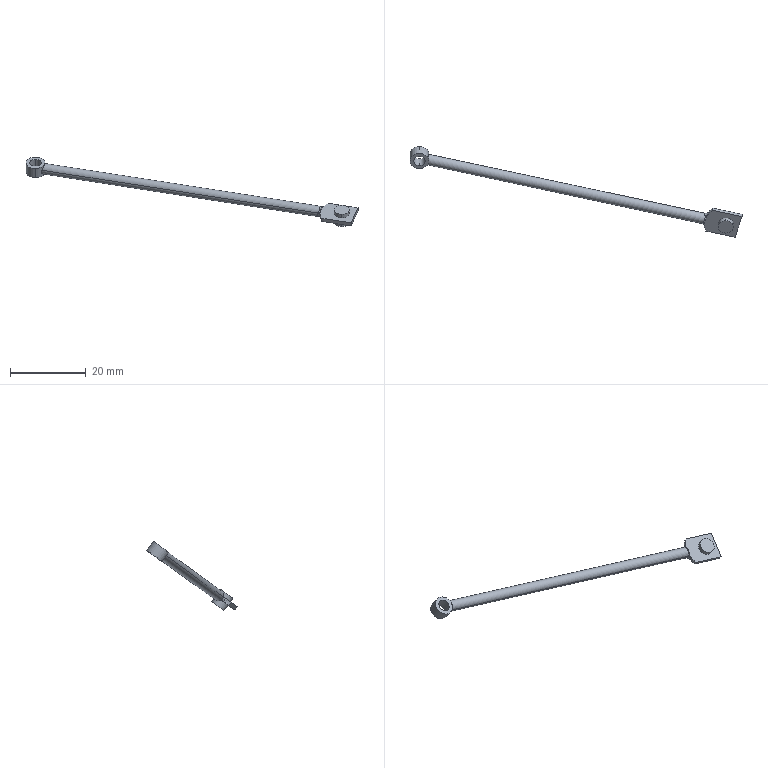Part | STEP file | Completa.sldasm-Part-145_Valor predeterminado | 1 solid | 27 faces | box 87.747 x 23.93 x 18.349 mm | volume 604.413 mm3 | cylinder 14 | plane 9 | spline 4 | commonest cylinder face diameters 4 x4 11.4 x4 2.8 x2 3 x2 5 x2